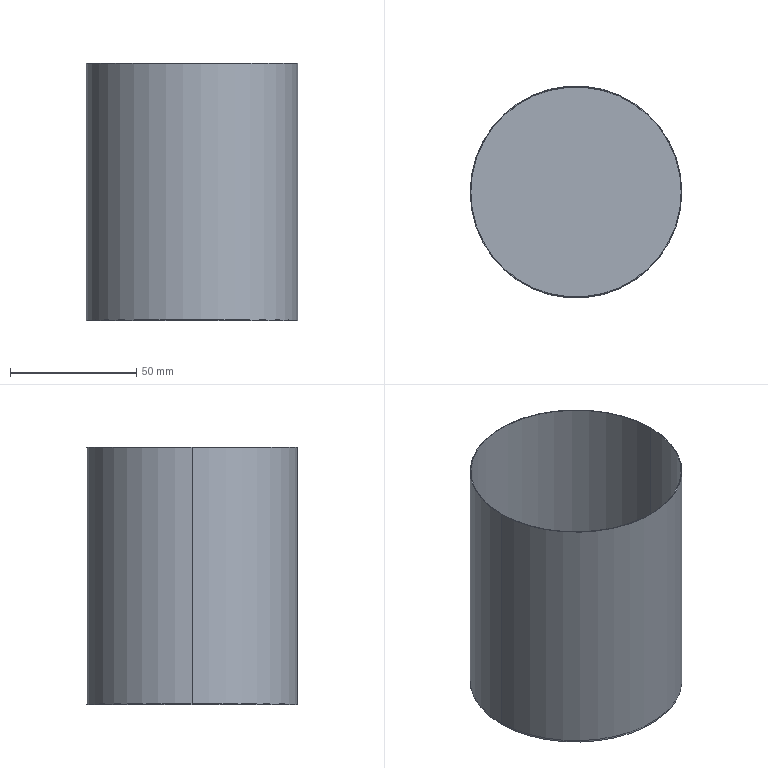Part | SolidWorks | features BaseBody 1 | 1 solid | 7 faces | box 84 x 84 x 102 mm | volume 9447 mm3 | cylinder 4 | plane 3 | commonest cylinder face diameters 83.5 x2 84 x2
STEP:
#1=CARTESIAN_POINT('',(-42.,0.,102.));
#2=VERTEX_POINT('',#1);
#3=CARTESIAN_POINT('',(42.,0.,102.));
#4=VERTEX_POINT('',#3);
#5=CARTESIAN_POINT('',(0.,0.,102.));
#6=DIRECTION('',(0.,0.,-1.));
#7=DIRECTION('',(-1.,0.,0.));
#8=AXIS2_PLACEMENT_3D('',#5,#6,#7);
#9=CIRCLE('',#8,42.);
#10=EDGE_CURVE('',#2,#4,#9,.T.);
#11=ORIENTED_EDGE('',*,*,#10,.T.);
#12=CARTESIAN_POINT('',(42.,0.,0.));
#13=VERTEX_POINT('',#12);
#14=CARTESIAN_POINT('',(42.,0.,102.));
#15=DIRECTION('',(0.,0.,-1.));
#16=VECTOR('',#15,1000.);
#17=LINE('',#14,#16);
#18=EDGE_CURVE('',#4,#13,#17,.T.);
#19=ORIENTED_EDGE('',*,*,#18,.T.);
#20=CARTESIAN_POINT('',(-42.,0.,0.));
#21=VERTEX_POINT('',#20);
#22=CARTESIAN_POINT('',(0.,0.,0.));
#23=DIRECTION('',(0.,0.,1.));
#24=DIRECTION('',(-1.,0.,0.));
#25=AXIS2_PLACEMENT_3D('',#22,#23,#24);
#26=CIRCLE('',#25,42.);
#27=EDGE_CURVE('',#13,#21,#26,.T.);
#28=ORIENTED_EDGE('',*,*,#27,.T.);
#29=CARTESIAN_POINT('',(-42.,0.,102.));
#30=DIRECTION('',(0.,0.,-1.));
#31=VECTOR('',#30,1000.);
#32=LINE('',#29,#31);
#33=EDGE_CURVE('',#2,#21,#32,.T.);
#34=ORIENTED_EDGE('',*,*,#33,.F.);
#35=EDGE_LOOP('',(#11,#19,#28,#34));
#36=FACE_OUTER_BOUND('',#35,.T.);
#37=CARTESIAN_POINT('',(0.,0.,102.));
#38=DIRECTION('',(0.,0.,-1.));
#39=DIRECTION('',(-1.,0.,0.));
#40=AXIS2_PLACEMENT_3D('',#37,#38,#39);
#41=CYLINDRICAL_SURFACE('',#40,42.);
#42=ADVANCED_FACE('',(#36),#41,.T.);
#43=CARTESIAN_POINT('',(41.75,0.,102.));
#44=VERTEX_POINT('',#43);
#45=CARTESIAN_POINT('',(-41.75,0.,102.));
#46=VERTEX_POINT('',#45);
#47=CARTESIAN_POINT('',(0.,0.,102.));
#48=DIRECTION('',(0.,0.,-1.));
#49=DIRECTION('',(-1.,0.,0.));
#50=AXIS2_PLACEMENT_3D('',#47,#48,#49);
#51=CIRCLE('',#50,41.75);
#52=EDGE_CURVE('',#44,#46,#51,.T.);
#53=ORIENTED_EDGE('',*,*,#52,.F.);
#54=CARTESIAN_POINT('',(41.75,0.,0.5));
#55=VERTEX_POINT('',#54);
#56=CARTESIAN_POINT('',(41.75,0.,102.));
#57=DIRECTION('',(0.,0.,-1.));
#58=VECTOR('',#57,1000.);
#59=LINE('',#56,#58);
#60=EDGE_CURVE('',#44,#55,#59,.T.);
#61=ORIENTED_EDGE('',*,*,#60,.T.);
#62=CARTESIAN_POINT('',(-41.75,0.,0.5));
#63=VERTEX_POINT('',#62);
#64=CARTESIAN_POINT('',(0.,0.,0.5));
#65=DIRECTION('',(0.,0.,1.));
#66=DIRECTION('',(-1.,0.,0.));
#67=AXIS2_PLACEMENT_3D('',#64,#65,#66);
#68=CIRCLE('',#67,41.75);
#69=EDGE_CURVE('',#63,#55,#68,.T.);
#70=ORIENTED_EDGE('',*,*,#69,.F.);
#71=CARTESIAN_POINT('',(-41.75,0.,102.));
#72=DIRECTION('',(0.,0.,-1.));
#73=VECTOR('',#72,1000.);
#74=LINE('',#71,#73);
#75=EDGE_CURVE('',#46,#63,#74,.T.);
#76=ORIENTED_EDGE('',*,*,#75,.F.);
#77=EDGE_LOOP('',(#53,#61,#70,#76));
#78=FACE_OUTER_BOUND('',#77,.T.);
#79=CARTESIAN_POINT('',(0.,0.,102.));
#80=DIRECTION('',(0.,0.,-1.));
#81=DIRECTION('',(-1.,0.,0.));
#82=AXIS2_PLACEMENT_3D('',#79,#80,#81);
#83=CYLINDRICAL_SURFACE('',#82,41.75);
#84=ADVANCED_FACE('',(#78),#83,.F.);
#85=ORIENTED_EDGE('',*,*,#18,.F.);
#86=CARTESIAN_POINT('',(0.,0.,102.));
#87=DIRECTION('',(0.,0.,-1.));
#88=DIRECTION('',(-1.,0.,0.));
#89=AXIS2_PLACEMENT_3D('',#86,#87,#88);
#90=CIRCLE('',#89,42.);
#91=EDGE_CURVE('',#4,#2,#90,.T.);
#92=ORIENTED_EDGE('',*,*,#91,.T.);
#93=ORIENTED_EDGE('',*,*,#33,.T.);
#94=CARTESIAN_POINT('',(0.,0.,0.));
#95=DIRECTION('',(0.,0.,1.));
#96=DIRECTION('',(-1.,0.,0.));
#97=AXIS2_PLACEMENT_3D('',#94,#95,#96);
#98=CIRCLE('',#97,42.);
#99=EDGE_CURVE('',#21,#13,#98,.T.);
#100=ORIENTED_EDGE('',*,*,#99,.T.);
#101=EDGE_LOOP('',(#85,#92,#93,#100));
#102=FACE_OUTER_BOUND('',#101,.T.);
#103=CARTESIAN_POINT('',(0.,0.,102.));
#104=DIRECTION('',(0.,0.,-1.));
#105=DIRECTION('',(-1.,0.,0.));
#106=AXIS2_PLACEMENT_3D('',#103,#104,#105);
#107=CYLINDRICAL_SURFACE('',#106,42.);
#108=ADVANCED_FACE('',(#102),#107,.T.);
#109=ORIENTED_EDGE('',*,*,#99,.F.);
#110=ORIENTED_EDGE('',*,*,#27,.F.);
#111=EDGE_LOOP('',(#109,#110));
#112=FACE_OUTER_BOUND('',#111,.T.);
#113=CARTESIAN_POINT('',(0.,0.,0.));
#114=DIRECTION('',(0.,0.,1.));
#115=DIRECTION('',(1.,0.,0.));
#116=AXIS2_PLACEMENT_3D('',#113,#114,#115);
#117=PLANE('',#116);
#118=ADVANCED_FACE('',(#112),#117,.F.);
#119=CARTESIAN_POINT('',(0.,0.,102.));
#120=DIRECTION('',(0.,0.,-1.));
#121=DIRECTION('',(-1.,0.,0.));
#122=AXIS2_PLACEMENT_3D('',#119,#120,#121);
#123=CIRCLE('',#122,41.75);
#124=EDGE_CURVE('',#46,#44,#123,.T.);
#125=ORIENTED_EDGE('',*,*,#124,.T.);
#126=ORIENTED_EDGE('',*,*,#52,.T.);
#127=EDGE_LOOP('',(#125,#126));
#128=FACE_BOUND('',#127,.T.);
#129=ORIENTED_EDGE('',*,*,#10,.F.);
#130=ORIENTED_EDGE('',*,*,#91,.F.);
#131=EDGE_LOOP('',(#129,#130));
#132=FACE_OUTER_BOUND('',#131,.T.);
#133=CARTESIAN_POINT('',(0.,0.,102.));
#134=DIRECTION('',(0.,0.,1.));
#135=DIRECTION('',(1.,0.,0.));
#136=AXIS2_PLACEMENT_3D('',#133,#134,#135);
#137=PLANE('',#136);
#138=ADVANCED_FACE('',(#128,#132),#137,.T.);
#139=ORIENTED_EDGE('',*,*,#60,.F.);
#140=ORIENTED_EDGE('',*,*,#124,.F.);
#141=ORIENTED_EDGE('',*,*,#75,.T.);
#142=CARTESIAN_POINT('',(0.,0.,0.5));
#143=DIRECTION('',(0.,0.,1.));
#144=DIRECTION('',(-1.,0.,0.));
#145=AXIS2_PLACEMENT_3D('',#142,#143,#144);
#146=CIRCLE('',#145,41.75);
#147=EDGE_CURVE('',#55,#63,#146,.T.);
#148=ORIENTED_EDGE('',*,*,#147,.F.);
#149=EDGE_LOOP('',(#139,#140,#141,#148));
#150=FACE_OUTER_BOUND('',#149,.T.);
#151=CARTESIAN_POINT('',(0.,0.,102.));
#152=DIRECTION('',(0.,0.,-1.));
#153=DIRECTION('',(-1.,0.,0.));
#154=AXIS2_PLACEMENT_3D('',#151,#152,#153);
#155=CYLINDRICAL_SURFACE('',#154,41.75);
#156=ADVANCED_FACE('',(#150),#155,.F.);
#157=ORIENTED_EDGE('',*,*,#69,.T.);
#158=ORIENTED_EDGE('',*,*,#147,.T.);
#159=EDGE_LOOP('',(#157,#158));
#160=FACE_OUTER_BOUND('',#159,.T.);
#161=CARTESIAN_POINT('',(0.,0.,0.5));
#162=DIRECTION('',(0.,0.,-1.));
#163=DIRECTION('',(-1.,0.,0.));
#164=AXIS2_PLACEMENT_3D('',#161,#162,#163);
#165=PLANE('',#164);
#166=ADVANCED_FACE('',(#160),#165,.F.);
#167=CLOSED_SHELL('',(#42,#84,#108,#118,#138,#156,#166));
#168=MANIFOLD_SOLID_BREP('',#167);
#169=CARTESIAN_POINT('',(0.,0.,0.));
#170=DIRECTION('',(0.,0.,1.));
#171=DIRECTION('',(1.,0.,0.));
#172=AXIS2_PLACEMENT_3D('',#169,#170,#171);
#173=(LENGTH_UNIT()NAMED_UNIT(*)SI_UNIT(.MILLI.,.METRE.));
#174=UNCERTAINTY_MEASURE_WITH_UNIT(LENGTH_MEASURE(0.00001),#173,'','');
#175=(NAMED_UNIT(*)PLANE_ANGLE_UNIT()SI_UNIT($,.RADIAN.));
#176=(NAMED_UNIT(*)SI_UNIT($,.STERADIAN.)SOLID_ANGLE_UNIT());
#177=(GEOMETRIC_REPRESENTATION_CONTEXT(3)GLOBAL_UNCERTAINTY_ASSIGNED_CONTEXT((#174))GLOBAL_UNIT_ASSIGNED_CONTEXT((#173,#175,#176))REPRESENTATION_CONTEXT('',''));
#178=ADVANCED_BREP_SHAPE_REPRESENTATION('',(#168,#172),#177);